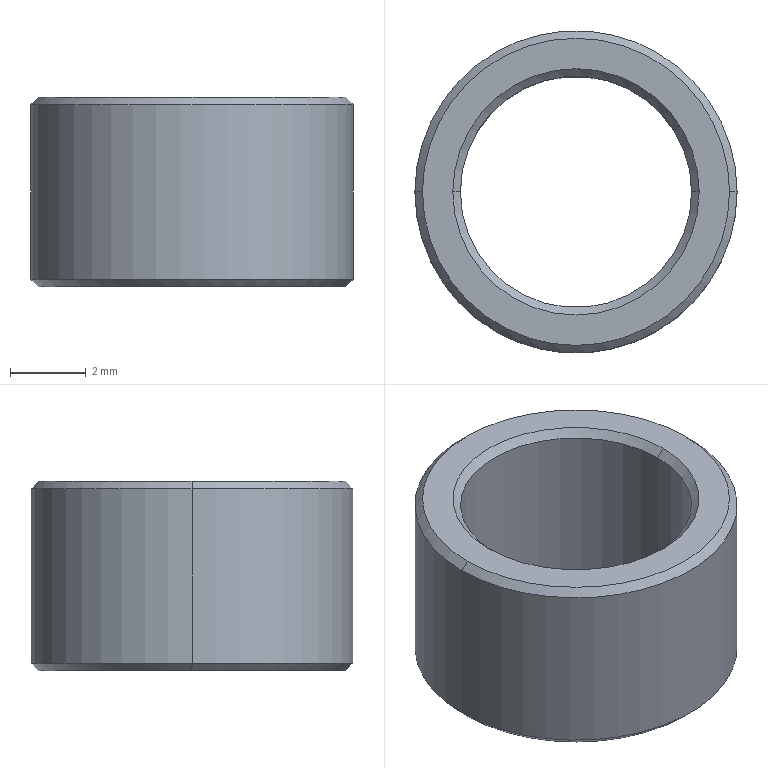Part | NX | features BREP 1 | 1 solid | 14 faces | box 8.5 x 8.5 x 5 mm | volume 135.767 mm3 | cone 8 | cylinder 4 | plane 2 | commonest cylinder face diameters 6.1 x2 8.5 x2
STEP:
#1=CARTESIAN_POINT('',(-3.25,0.,5.));
#2=VERTEX_POINT('',#1);
#3=CARTESIAN_POINT('',(-3.05,0.,4.8));
#4=VERTEX_POINT('',#3);
#5=CARTESIAN_POINT('',(-3.05,0.,4.8));
#6=DIRECTION('',(-0.7071,0.,0.7071));
#7=VECTOR('',#6,1000.);
#8=LINE('',#5,#7);
#9=EDGE_CURVE('',#2,#4,#8,.F.);
#10=ORIENTED_EDGE('',*,*,#9,.T.);
#11=CARTESIAN_POINT('',(3.05,0.,4.8));
#12=VERTEX_POINT('',#11);
#13=CARTESIAN_POINT('',(0.,0.,4.8));
#14=DIRECTION('',(0.,0.,1.));
#15=DIRECTION('',(1.,0.,0.));
#16=AXIS2_PLACEMENT_3D('',#13,#14,#15);
#17=CIRCLE('',#16,3.05);
#18=EDGE_CURVE('',#12,#4,#17,.T.);
#19=ORIENTED_EDGE('',*,*,#18,.F.);
#20=CARTESIAN_POINT('',(3.25,0.,5.));
#21=VERTEX_POINT('',#20);
#22=CARTESIAN_POINT('',(3.05,0.,4.8));
#23=DIRECTION('',(0.7071,0.,0.7071));
#24=VECTOR('',#23,1000.);
#25=LINE('',#22,#24);
#26=EDGE_CURVE('',#21,#12,#25,.F.);
#27=ORIENTED_EDGE('',*,*,#26,.F.);
#28=CARTESIAN_POINT('',(0.,0.,5.));
#29=DIRECTION('',(0.,0.,-1.));
#30=DIRECTION('',(1.,0.,0.));
#31=AXIS2_PLACEMENT_3D('',#28,#29,#30);
#32=CIRCLE('',#31,3.25);
#33=EDGE_CURVE('',#2,#21,#32,.T.);
#34=ORIENTED_EDGE('',*,*,#33,.F.);
#35=EDGE_LOOP('',(#10,#19,#27,#34));
#36=FACE_BOUND('',#35,.T.);
#37=CARTESIAN_POINT('',(0.,0.,4.8));
#38=DIRECTION('',(0.,0.,1.));
#39=DIRECTION('',(1.,0.,0.));
#40=AXIS2_PLACEMENT_3D('',#37,#38,#39);
#41=CONICAL_SURFACE('',#40,3.05,0.7854);
#42=ADVANCED_FACE('',(#36),#41,.F.);
#43=CARTESIAN_POINT('',(4.05,0.,5.));
#44=VERTEX_POINT('',#43);
#45=CARTESIAN_POINT('',(4.25,0.,4.8));
#46=VERTEX_POINT('',#45);
#47=CARTESIAN_POINT('',(4.05,0.,5.));
#48=DIRECTION('',(0.7071,0.,-0.7071));
#49=VECTOR('',#48,1000.);
#50=LINE('',#47,#49);
#51=EDGE_CURVE('',#44,#46,#50,.T.);
#52=ORIENTED_EDGE('',*,*,#51,.F.);
#53=CARTESIAN_POINT('',(-4.05,0.,5.));
#54=VERTEX_POINT('',#53);
#55=CARTESIAN_POINT('',(0.,0.,5.));
#56=DIRECTION('',(0.,0.,1.));
#57=DIRECTION('',(1.,0.,0.));
#58=AXIS2_PLACEMENT_3D('',#55,#56,#57);
#59=CIRCLE('',#58,4.05);
#60=EDGE_CURVE('',#54,#44,#59,.T.);
#61=ORIENTED_EDGE('',*,*,#60,.F.);
#62=CARTESIAN_POINT('',(-4.25,0.,4.8));
#63=VERTEX_POINT('',#62);
#64=CARTESIAN_POINT('',(-4.05,0.,5.));
#65=DIRECTION('',(-0.7071,0.,-0.7071));
#66=VECTOR('',#65,1000.);
#67=LINE('',#64,#66);
#68=EDGE_CURVE('',#54,#63,#67,.T.);
#69=ORIENTED_EDGE('',*,*,#68,.T.);
#70=CARTESIAN_POINT('',(0.,0.,4.8));
#71=DIRECTION('',(0.,0.,-1.));
#72=DIRECTION('',(1.,0.,0.));
#73=AXIS2_PLACEMENT_3D('',#70,#71,#72);
#74=CIRCLE('',#73,4.25);
#75=EDGE_CURVE('',#46,#63,#74,.T.);
#76=ORIENTED_EDGE('',*,*,#75,.F.);
#77=EDGE_LOOP('',(#52,#61,#69,#76));
#78=FACE_BOUND('',#77,.T.);
#79=CARTESIAN_POINT('',(0.,0.,5.));
#80=DIRECTION('',(0.,0.,-1.));
#81=DIRECTION('',(-1.,0.,0.));
#82=AXIS2_PLACEMENT_3D('',#79,#80,#81);
#83=CONICAL_SURFACE('',#82,4.05,0.7854);
#84=ADVANCED_FACE('',(#78),#83,.T.);
#85=CARTESIAN_POINT('',(-4.25,0.,0.2));
#86=VERTEX_POINT('',#85);
#87=CARTESIAN_POINT('',(-4.05,0.,0.));
#88=VERTEX_POINT('',#87);
#89=CARTESIAN_POINT('',(-4.25,0.,0.2));
#90=DIRECTION('',(-0.7071,0.,0.7071));
#91=VECTOR('',#90,1000.);
#92=LINE('',#89,#91);
#93=EDGE_CURVE('',#86,#88,#92,.F.);
#94=ORIENTED_EDGE('',*,*,#93,.T.);
#95=CARTESIAN_POINT('',(4.05,0.,0.));
#96=VERTEX_POINT('',#95);
#97=CARTESIAN_POINT('',(0.,0.,0.));
#98=DIRECTION('',(0.,0.,-1.));
#99=DIRECTION('',(1.,0.,0.));
#100=AXIS2_PLACEMENT_3D('',#97,#98,#99);
#101=CIRCLE('',#100,4.05);
#102=EDGE_CURVE('',#96,#88,#101,.T.);
#103=ORIENTED_EDGE('',*,*,#102,.F.);
#104=CARTESIAN_POINT('',(4.25,0.,0.2));
#105=VERTEX_POINT('',#104);
#106=CARTESIAN_POINT('',(4.25,0.,0.2));
#107=DIRECTION('',(0.7071,0.,0.7071));
#108=VECTOR('',#107,1000.);
#109=LINE('',#106,#108);
#110=EDGE_CURVE('',#105,#96,#109,.F.);
#111=ORIENTED_EDGE('',*,*,#110,.F.);
#112=CARTESIAN_POINT('',(0.,0.,0.2));
#113=DIRECTION('',(0.,0.,1.));
#114=DIRECTION('',(1.,0.,0.));
#115=AXIS2_PLACEMENT_3D('',#112,#113,#114);
#116=CIRCLE('',#115,4.25);
#117=EDGE_CURVE('',#86,#105,#116,.T.);
#118=ORIENTED_EDGE('',*,*,#117,.F.);
#119=EDGE_LOOP('',(#94,#103,#111,#118));
#120=FACE_BOUND('',#119,.T.);
#121=CARTESIAN_POINT('',(0.,0.,0.2));
#122=DIRECTION('',(0.,0.,1.));
#123=DIRECTION('',(1.,0.,0.));
#124=AXIS2_PLACEMENT_3D('',#121,#122,#123);
#125=CONICAL_SURFACE('',#124,4.25,0.7854);
#126=ADVANCED_FACE('',(#120),#125,.T.);
#127=CARTESIAN_POINT('',(3.05,0.,0.2));
#128=VERTEX_POINT('',#127);
#129=CARTESIAN_POINT('',(3.25,0.,0.));
#130=VERTEX_POINT('',#129);
#131=CARTESIAN_POINT('',(3.25,0.,0.));
#132=DIRECTION('',(0.7071,0.,-0.7071));
#133=VECTOR('',#132,1000.);
#134=LINE('',#131,#133);
#135=EDGE_CURVE('',#128,#130,#134,.T.);
#136=ORIENTED_EDGE('',*,*,#135,.F.);
#137=CARTESIAN_POINT('',(-3.05,0.,0.2));
#138=VERTEX_POINT('',#137);
#139=CARTESIAN_POINT('',(0.,0.,0.2));
#140=DIRECTION('',(0.,0.,-1.));
#141=DIRECTION('',(1.,0.,0.));
#142=AXIS2_PLACEMENT_3D('',#139,#140,#141);
#143=CIRCLE('',#142,3.05);
#144=EDGE_CURVE('',#138,#128,#143,.T.);
#145=ORIENTED_EDGE('',*,*,#144,.F.);
#146=CARTESIAN_POINT('',(-3.25,0.,0.));
#147=VERTEX_POINT('',#146);
#148=CARTESIAN_POINT('',(-3.25,0.,0.));
#149=DIRECTION('',(-0.7071,0.,-0.7071));
#150=VECTOR('',#149,1000.);
#151=LINE('',#148,#150);
#152=EDGE_CURVE('',#138,#147,#151,.T.);
#153=ORIENTED_EDGE('',*,*,#152,.T.);
#154=CARTESIAN_POINT('',(0.,0.,0.));
#155=DIRECTION('',(0.,0.,1.));
#156=DIRECTION('',(1.,0.,0.));
#157=AXIS2_PLACEMENT_3D('',#154,#155,#156);
#158=CIRCLE('',#157,3.25);
#159=EDGE_CURVE('',#130,#147,#158,.T.);
#160=ORIENTED_EDGE('',*,*,#159,.F.);
#161=EDGE_LOOP('',(#136,#145,#153,#160));
#162=FACE_BOUND('',#161,.T.);
#163=CARTESIAN_POINT('',(0.,0.,0.));
#164=DIRECTION('',(0.,0.,-1.));
#165=DIRECTION('',(-1.,0.,0.));
#166=AXIS2_PLACEMENT_3D('',#163,#164,#165);
#167=CONICAL_SURFACE('',#166,3.25,0.7854);
#168=ADVANCED_FACE('',(#162),#167,.F.);
#169=CARTESIAN_POINT('',(3.05,0.,5.));
#170=DIRECTION('',(0.,0.,-1.));
#171=VECTOR('',#170,1000.);
#172=LINE('',#169,#171);
#173=EDGE_CURVE('',#12,#128,#172,.T.);
#174=ORIENTED_EDGE('',*,*,#173,.F.);
#175=ORIENTED_EDGE('',*,*,#18,.T.);
#176=CARTESIAN_POINT('',(-3.05,0.,5.));
#177=DIRECTION('',(0.,0.,-1.));
#178=VECTOR('',#177,1000.);
#179=LINE('',#176,#178);
#180=EDGE_CURVE('',#4,#138,#179,.T.);
#181=ORIENTED_EDGE('',*,*,#180,.T.);
#182=ORIENTED_EDGE('',*,*,#144,.T.);
#183=EDGE_LOOP('',(#174,#175,#181,#182));
#184=FACE_BOUND('',#183,.T.);
#185=CARTESIAN_POINT('',(0.,0.,5.));
#186=DIRECTION('',(0.,0.,-1.));
#187=DIRECTION('',(-1.,0.,0.));
#188=AXIS2_PLACEMENT_3D('',#185,#186,#187);
#189=CYLINDRICAL_SURFACE('',#188,3.05);
#190=ADVANCED_FACE('',(#184),#189,.F.);
#191=CARTESIAN_POINT('',(4.25,0.,5.));
#192=DIRECTION('',(0.,0.,-1.));
#193=VECTOR('',#192,1000.);
#194=LINE('',#191,#193);
#195=EDGE_CURVE('',#46,#105,#194,.T.);
#196=ORIENTED_EDGE('',*,*,#195,.F.);
#197=ORIENTED_EDGE('',*,*,#75,.T.);
#198=CARTESIAN_POINT('',(-4.25,0.,5.));
#199=DIRECTION('',(0.,0.,-1.));
#200=VECTOR('',#199,1000.);
#201=LINE('',#198,#200);
#202=EDGE_CURVE('',#63,#86,#201,.T.);
#203=ORIENTED_EDGE('',*,*,#202,.T.);
#204=ORIENTED_EDGE('',*,*,#117,.T.);
#205=EDGE_LOOP('',(#196,#197,#203,#204));
#206=FACE_BOUND('',#205,.T.);
#207=CARTESIAN_POINT('',(0.,0.,5.));
#208=DIRECTION('',(0.,0.,-1.));
#209=DIRECTION('',(-1.,0.,0.));
#210=AXIS2_PLACEMENT_3D('',#207,#208,#209);
#211=CYLINDRICAL_SURFACE('',#210,4.25);
#212=ADVANCED_FACE('',(#206),#211,.T.);
#213=ORIENTED_EDGE('',*,*,#102,.T.);
#214=CARTESIAN_POINT('',(0.,0.,0.));
#215=DIRECTION('',(0.,0.,-1.));
#216=DIRECTION('',(1.,0.,0.));
#217=AXIS2_PLACEMENT_3D('',#214,#215,#216);
#218=CIRCLE('',#217,4.05);
#219=EDGE_CURVE('',#88,#96,#218,.T.);
#220=ORIENTED_EDGE('',*,*,#219,.T.);
#221=EDGE_LOOP('',(#213,#220));
#222=FACE_BOUND('',#221,.T.);
#223=CARTESIAN_POINT('',(0.,0.,0.));
#224=DIRECTION('',(0.,0.,1.));
#225=DIRECTION('',(1.,0.,0.));
#226=AXIS2_PLACEMENT_3D('',#223,#224,#225);
#227=CIRCLE('',#226,3.25);
#228=EDGE_CURVE('',#147,#130,#227,.T.);
#229=ORIENTED_EDGE('',*,*,#228,.T.);
#230=ORIENTED_EDGE('',*,*,#159,.T.);
#231=EDGE_LOOP('',(#229,#230));
#232=FACE_BOUND('',#231,.T.);
#233=CARTESIAN_POINT('',(0.,0.,0.));
#234=DIRECTION('',(0.,0.,1.));
#235=DIRECTION('',(1.,0.,0.));
#236=AXIS2_PLACEMENT_3D('',#233,#234,#235);
#237=PLANE('',#236);
#238=ADVANCED_FACE('',(#222,#232),#237,.F.);
#239=CARTESIAN_POINT('',(0.,0.,5.));
#240=DIRECTION('',(0.,0.,-1.));
#241=DIRECTION('',(1.,0.,0.));
#242=AXIS2_PLACEMENT_3D('',#239,#240,#241);
#243=CIRCLE('',#242,3.25);
#244=EDGE_CURVE('',#21,#2,#243,.T.);
#245=ORIENTED_EDGE('',*,*,#244,.T.);
#246=ORIENTED_EDGE('',*,*,#33,.T.);
#247=EDGE_LOOP('',(#245,#246));
#248=FACE_BOUND('',#247,.T.);
#249=ORIENTED_EDGE('',*,*,#60,.T.);
#250=CARTESIAN_POINT('',(0.,0.,5.));
#251=DIRECTION('',(0.,0.,1.));
#252=DIRECTION('',(1.,0.,0.));
#253=AXIS2_PLACEMENT_3D('',#250,#251,#252);
#254=CIRCLE('',#253,4.05);
#255=EDGE_CURVE('',#44,#54,#254,.T.);
#256=ORIENTED_EDGE('',*,*,#255,.T.);
#257=EDGE_LOOP('',(#249,#256));
#258=FACE_BOUND('',#257,.T.);
#259=CARTESIAN_POINT('',(0.,0.,5.));
#260=DIRECTION('',(0.,0.,1.));
#261=DIRECTION('',(1.,0.,0.));
#262=AXIS2_PLACEMENT_3D('',#259,#260,#261);
#263=PLANE('',#262);
#264=ADVANCED_FACE('',(#248,#258),#263,.T.);
#265=CARTESIAN_POINT('',(0.,0.,4.8));
#266=DIRECTION('',(0.,0.,-1.));
#267=DIRECTION('',(1.,0.,0.));
#268=AXIS2_PLACEMENT_3D('',#265,#266,#267);
#269=CIRCLE('',#268,4.25);
#270=EDGE_CURVE('',#63,#46,#269,.T.);
#271=ORIENTED_EDGE('',*,*,#270,.T.);
#272=ORIENTED_EDGE('',*,*,#195,.T.);
#273=CARTESIAN_POINT('',(0.,0.,0.2));
#274=DIRECTION('',(0.,0.,1.));
#275=DIRECTION('',(1.,0.,0.));
#276=AXIS2_PLACEMENT_3D('',#273,#274,#275);
#277=CIRCLE('',#276,4.25);
#278=EDGE_CURVE('',#105,#86,#277,.T.);
#279=ORIENTED_EDGE('',*,*,#278,.T.);
#280=ORIENTED_EDGE('',*,*,#202,.F.);
#281=EDGE_LOOP('',(#271,#272,#279,#280));
#282=FACE_BOUND('',#281,.T.);
#283=CARTESIAN_POINT('',(0.,0.,5.));
#284=DIRECTION('',(0.,0.,-1.));
#285=DIRECTION('',(-1.,0.,0.));
#286=AXIS2_PLACEMENT_3D('',#283,#284,#285);
#287=CYLINDRICAL_SURFACE('',#286,4.25);
#288=ADVANCED_FACE('',(#282),#287,.T.);
#289=CARTESIAN_POINT('',(0.,0.,4.8));
#290=DIRECTION('',(0.,0.,1.));
#291=DIRECTION('',(1.,0.,0.));
#292=AXIS2_PLACEMENT_3D('',#289,#290,#291);
#293=CIRCLE('',#292,3.05);
#294=EDGE_CURVE('',#4,#12,#293,.T.);
#295=ORIENTED_EDGE('',*,*,#294,.T.);
#296=ORIENTED_EDGE('',*,*,#173,.T.);
#297=CARTESIAN_POINT('',(0.,0.,0.2));
#298=DIRECTION('',(0.,0.,-1.));
#299=DIRECTION('',(1.,0.,0.));
#300=AXIS2_PLACEMENT_3D('',#297,#298,#299);
#301=CIRCLE('',#300,3.05);
#302=EDGE_CURVE('',#128,#138,#301,.T.);
#303=ORIENTED_EDGE('',*,*,#302,.T.);
#304=ORIENTED_EDGE('',*,*,#180,.F.);
#305=EDGE_LOOP('',(#295,#296,#303,#304));
#306=FACE_BOUND('',#305,.T.);
#307=CARTESIAN_POINT('',(0.,0.,5.));
#308=DIRECTION('',(0.,0.,-1.));
#309=DIRECTION('',(-1.,0.,0.));
#310=AXIS2_PLACEMENT_3D('',#307,#308,#309);
#311=CYLINDRICAL_SURFACE('',#310,3.05);
#312=ADVANCED_FACE('',(#306),#311,.F.);
#313=ORIENTED_EDGE('',*,*,#302,.F.);
#314=ORIENTED_EDGE('',*,*,#135,.T.);
#315=ORIENTED_EDGE('',*,*,#228,.F.);
#316=ORIENTED_EDGE('',*,*,#152,.F.);
#317=EDGE_LOOP('',(#313,#314,#315,#316));
#318=FACE_BOUND('',#317,.T.);
#319=CARTESIAN_POINT('',(0.,0.,0.));
#320=DIRECTION('',(0.,0.,-1.));
#321=DIRECTION('',(-1.,0.,0.));
#322=AXIS2_PLACEMENT_3D('',#319,#320,#321);
#323=CONICAL_SURFACE('',#322,3.25,0.7854);
#324=ADVANCED_FACE('',(#318),#323,.F.);
#325=ORIENTED_EDGE('',*,*,#219,.F.);
#326=ORIENTED_EDGE('',*,*,#93,.F.);
#327=ORIENTED_EDGE('',*,*,#278,.F.);
#328=ORIENTED_EDGE('',*,*,#110,.T.);
#329=EDGE_LOOP('',(#325,#326,#327,#328));
#330=FACE_BOUND('',#329,.T.);
#331=CARTESIAN_POINT('',(0.,0.,0.2));
#332=DIRECTION('',(0.,0.,1.));
#333=DIRECTION('',(1.,0.,0.));
#334=AXIS2_PLACEMENT_3D('',#331,#332,#333);
#335=CONICAL_SURFACE('',#334,4.25,0.7854);
#336=ADVANCED_FACE('',(#330),#335,.T.);
#337=ORIENTED_EDGE('',*,*,#255,.F.);
#338=ORIENTED_EDGE('',*,*,#51,.T.);
#339=ORIENTED_EDGE('',*,*,#270,.F.);
#340=ORIENTED_EDGE('',*,*,#68,.F.);
#341=EDGE_LOOP('',(#337,#338,#339,#340));
#342=FACE_BOUND('',#341,.T.);
#343=CARTESIAN_POINT('',(0.,0.,5.));
#344=DIRECTION('',(0.,0.,-1.));
#345=DIRECTION('',(-1.,0.,0.));
#346=AXIS2_PLACEMENT_3D('',#343,#344,#345);
#347=CONICAL_SURFACE('',#346,4.05,0.7854);
#348=ADVANCED_FACE('',(#342),#347,.T.);
#349=ORIENTED_EDGE('',*,*,#294,.F.);
#350=ORIENTED_EDGE('',*,*,#9,.F.);
#351=ORIENTED_EDGE('',*,*,#244,.F.);
#352=ORIENTED_EDGE('',*,*,#26,.T.);
#353=EDGE_LOOP('',(#349,#350,#351,#352));
#354=FACE_BOUND('',#353,.T.);
#355=CARTESIAN_POINT('',(0.,0.,4.8));
#356=DIRECTION('',(0.,0.,1.));
#357=DIRECTION('',(1.,0.,0.));
#358=AXIS2_PLACEMENT_3D('',#355,#356,#357);
#359=CONICAL_SURFACE('',#358,3.05,0.7854);
#360=ADVANCED_FACE('',(#354),#359,.F.);
#361=CLOSED_SHELL('',(#42,#84,#126,#168,#190,#212,#238,#264,#288,#312,#324,#336,#348,#360));
#362=MANIFOLD_SOLID_BREP('',#361);
#363=(LENGTH_UNIT()NAMED_UNIT(*)SI_UNIT(.MILLI.,.METRE.));
#364=UNCERTAINTY_MEASURE_WITH_UNIT(LENGTH_MEASURE(0.00001),#363,'','');
#365=(NAMED_UNIT(*)PLANE_ANGLE_UNIT()SI_UNIT($,.RADIAN.));
#366=(NAMED_UNIT(*)SI_UNIT($,.STERADIAN.)SOLID_ANGLE_UNIT());
#367=(GEOMETRIC_REPRESENTATION_CONTEXT(3)GLOBAL_UNCERTAINTY_ASSIGNED_CONTEXT((#364))GLOBAL_UNIT_ASSIGNED_CONTEXT((#363,#365,#366))REPRESENTATION_CONTEXT('',''));
#368=ADVANCED_BREP_SHAPE_REPRESENTATION('',(#362),#367);